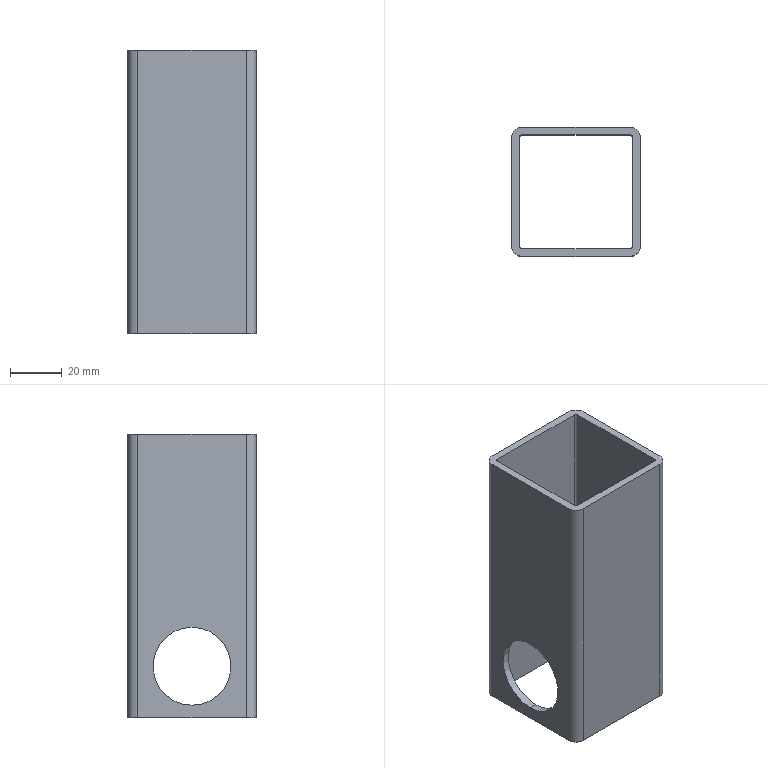Part | SolidWorks | features ExtruThin 1, ICE 1 | 1 solid | 22 faces | box 50 x 50 x 110 mm | volume 56326 mm3 | cylinder 12 | plane 10 | commonest cylinder face diameters 2 x4 8 x4 30.2 x4
STEP:
#1=CARTESIAN_POINT('',(22.,0.,4.9));
#2=VERTEX_POINT('',#1);
#3=CARTESIAN_POINT('',(22.,0.,35.1));
#4=VERTEX_POINT('',#3);
#5=CARTESIAN_POINT('',(22.,0.,20.));
#6=DIRECTION('',(-1.,0.,0.));
#7=DIRECTION('',(0.,0.,1.));
#8=AXIS2_PLACEMENT_3D('',#5,#6,#7);
#9=CIRCLE('',#8,15.1);
#10=EDGE_CURVE('',#2,#4,#9,.T.);
#11=ORIENTED_EDGE('',*,*,#10,.T.);
#12=CARTESIAN_POINT('',(25.,0.,35.1));
#13=VERTEX_POINT('',#12);
#14=CARTESIAN_POINT('',(-25.,0.,35.1));
#15=DIRECTION('',(1.,0.,0.));
#16=VECTOR('',#15,1000.);
#17=LINE('',#14,#16);
#18=EDGE_CURVE('',#4,#13,#17,.T.);
#19=ORIENTED_EDGE('',*,*,#18,.T.);
#20=CARTESIAN_POINT('',(25.,0.,4.9));
#21=VERTEX_POINT('',#20);
#22=CARTESIAN_POINT('',(25.,0.,20.));
#23=DIRECTION('',(1.,0.,0.));
#24=DIRECTION('',(0.,0.,-1.));
#25=AXIS2_PLACEMENT_3D('',#22,#23,#24);
#26=CIRCLE('',#25,15.1);
#27=EDGE_CURVE('',#13,#21,#26,.T.);
#28=ORIENTED_EDGE('',*,*,#27,.T.);
#29=CARTESIAN_POINT('',(-25.,0.,4.9));
#30=DIRECTION('',(1.,0.,0.));
#31=VECTOR('',#30,1000.);
#32=LINE('',#29,#31);
#33=EDGE_CURVE('',#2,#21,#32,.T.);
#34=ORIENTED_EDGE('',*,*,#33,.F.);
#35=EDGE_LOOP('',(#11,#19,#28,#34));
#36=FACE_OUTER_BOUND('',#35,.T.);
#37=CARTESIAN_POINT('',(-25.,0.,20.));
#38=DIRECTION('',(1.,0.,0.));
#39=DIRECTION('',(0.,0.,-1.));
#40=AXIS2_PLACEMENT_3D('',#37,#38,#39);
#41=CYLINDRICAL_SURFACE('',#40,15.1);
#42=ADVANCED_FACE('',(#36),#41,.F.);
#43=CARTESIAN_POINT('',(-25.,0.,35.1));
#44=VERTEX_POINT('',#43);
#45=CARTESIAN_POINT('',(-25.,0.,4.9));
#46=VERTEX_POINT('',#45);
#47=CARTESIAN_POINT('',(-25.,0.,20.));
#48=DIRECTION('',(1.,0.,0.));
#49=DIRECTION('',(0.,0.,-1.));
#50=AXIS2_PLACEMENT_3D('',#47,#48,#49);
#51=CIRCLE('',#50,15.1);
#52=EDGE_CURVE('',#44,#46,#51,.T.);
#53=ORIENTED_EDGE('',*,*,#52,.F.);
#54=CARTESIAN_POINT('',(-22.,0.,35.1));
#55=VERTEX_POINT('',#54);
#56=CARTESIAN_POINT('',(-25.,0.,35.1));
#57=DIRECTION('',(1.,0.,0.));
#58=VECTOR('',#57,1000.);
#59=LINE('',#56,#58);
#60=EDGE_CURVE('',#44,#55,#59,.T.);
#61=ORIENTED_EDGE('',*,*,#60,.T.);
#62=CARTESIAN_POINT('',(-22.,0.,4.9));
#63=VERTEX_POINT('',#62);
#64=CARTESIAN_POINT('',(-22.,0.,20.));
#65=DIRECTION('',(1.,0.,0.));
#66=DIRECTION('',(0.,0.,-1.));
#67=AXIS2_PLACEMENT_3D('',#64,#65,#66);
#68=CIRCLE('',#67,15.1);
#69=EDGE_CURVE('',#55,#63,#68,.T.);
#70=ORIENTED_EDGE('',*,*,#69,.T.);
#71=CARTESIAN_POINT('',(-25.,0.,4.9));
#72=DIRECTION('',(1.,0.,0.));
#73=VECTOR('',#72,1000.);
#74=LINE('',#71,#73);
#75=EDGE_CURVE('',#46,#63,#74,.T.);
#76=ORIENTED_EDGE('',*,*,#75,.F.);
#77=EDGE_LOOP('',(#53,#61,#70,#76));
#78=FACE_OUTER_BOUND('',#77,.T.);
#79=CARTESIAN_POINT('',(-25.,0.,20.));
#80=DIRECTION('',(1.,0.,0.));
#81=DIRECTION('',(0.,0.,-1.));
#82=AXIS2_PLACEMENT_3D('',#79,#80,#81);
#83=CYLINDRICAL_SURFACE('',#82,15.1);
#84=ADVANCED_FACE('',(#78),#83,.F.);
#85=CARTESIAN_POINT('',(-25.,-21.,110.));
#86=VERTEX_POINT('',#85);
#87=CARTESIAN_POINT('',(-21.,-25.,110.));
#88=VERTEX_POINT('',#87);
#89=CARTESIAN_POINT('',(-21.,-21.,110.));
#90=DIRECTION('',(0.,0.,1.));
#91=DIRECTION('',(-1.,0.,0.));
#92=AXIS2_PLACEMENT_3D('',#89,#90,#91);
#93=CIRCLE('',#92,4.);
#94=EDGE_CURVE('',#86,#88,#93,.T.);
#95=ORIENTED_EDGE('',*,*,#94,.T.);
#96=CARTESIAN_POINT('',(21.,-25.,110.));
#97=VERTEX_POINT('',#96);
#98=CARTESIAN_POINT('',(-21.,-25.,110.));
#99=DIRECTION('',(1.,0.,0.));
#100=VECTOR('',#99,1000.);
#101=LINE('',#98,#100);
#102=EDGE_CURVE('',#88,#97,#101,.T.);
#103=ORIENTED_EDGE('',*,*,#102,.T.);
#104=CARTESIAN_POINT('',(25.,-21.,110.));
#105=VERTEX_POINT('',#104);
#106=CARTESIAN_POINT('',(21.,-21.,110.));
#107=DIRECTION('',(0.,0.,1.));
#108=DIRECTION('',(1.,0.,0.));
#109=AXIS2_PLACEMENT_3D('',#106,#107,#108);
#110=CIRCLE('',#109,4.);
#111=EDGE_CURVE('',#97,#105,#110,.T.);
#112=ORIENTED_EDGE('',*,*,#111,.T.);
#113=CARTESIAN_POINT('',(25.,21.,110.));
#114=VERTEX_POINT('',#113);
#115=CARTESIAN_POINT('',(25.,-21.,110.));
#116=DIRECTION('',(0.,1.,0.));
#117=VECTOR('',#116,1000.);
#118=LINE('',#115,#117);
#119=EDGE_CURVE('',#105,#114,#118,.T.);
#120=ORIENTED_EDGE('',*,*,#119,.T.);
#121=CARTESIAN_POINT('',(21.,25.,110.));
#122=VERTEX_POINT('',#121);
#123=CARTESIAN_POINT('',(21.,21.,110.));
#124=DIRECTION('',(0.,0.,1.));
#125=DIRECTION('',(-1.,0.,0.));
#126=AXIS2_PLACEMENT_3D('',#123,#124,#125);
#127=CIRCLE('',#126,4.);
#128=EDGE_CURVE('',#114,#122,#127,.T.);
#129=ORIENTED_EDGE('',*,*,#128,.T.);
#130=CARTESIAN_POINT('',(-21.,25.,110.));
#131=VERTEX_POINT('',#130);
#132=CARTESIAN_POINT('',(-21.,25.,110.));
#133=DIRECTION('',(-1.,0.,0.));
#134=VECTOR('',#133,1000.);
#135=LINE('',#132,#134);
#136=EDGE_CURVE('',#122,#131,#135,.T.);
#137=ORIENTED_EDGE('',*,*,#136,.T.);
#138=CARTESIAN_POINT('',(-25.,21.,110.));
#139=VERTEX_POINT('',#138);
#140=CARTESIAN_POINT('',(-21.,21.,110.));
#141=DIRECTION('',(0.,0.,1.));
#142=DIRECTION('',(-1.,0.,0.));
#143=AXIS2_PLACEMENT_3D('',#140,#141,#142);
#144=CIRCLE('',#143,4.);
#145=EDGE_CURVE('',#131,#139,#144,.T.);
#146=ORIENTED_EDGE('',*,*,#145,.T.);
#147=CARTESIAN_POINT('',(-25.,-21.,110.));
#148=DIRECTION('',(0.,-1.,0.));
#149=VECTOR('',#148,1000.);
#150=LINE('',#147,#149);
#151=EDGE_CURVE('',#139,#86,#150,.T.);
#152=ORIENTED_EDGE('',*,*,#151,.T.);
#153=EDGE_LOOP('',(#95,#103,#112,#120,#129,#137,#146,#152));
#154=FACE_OUTER_BOUND('',#153,.T.);
#155=CARTESIAN_POINT('',(-21.,-22.,110.));
#156=VERTEX_POINT('',#155);
#157=CARTESIAN_POINT('',(21.,-22.,110.));
#158=VERTEX_POINT('',#157);
#159=CARTESIAN_POINT('',(-21.,-22.,110.));
#160=DIRECTION('',(1.,0.,0.));
#161=VECTOR('',#160,1000.);
#162=LINE('',#159,#161);
#163=EDGE_CURVE('',#156,#158,#162,.T.);
#164=ORIENTED_EDGE('',*,*,#163,.F.);
#165=CARTESIAN_POINT('',(-22.,-21.,110.));
#166=VERTEX_POINT('',#165);
#167=CARTESIAN_POINT('',(-21.,-21.,110.));
#168=DIRECTION('',(0.,0.,1.));
#169=DIRECTION('',(-1.,0.,0.));
#170=AXIS2_PLACEMENT_3D('',#167,#168,#169);
#171=CIRCLE('',#170,1.);
#172=EDGE_CURVE('',#166,#156,#171,.T.);
#173=ORIENTED_EDGE('',*,*,#172,.F.);
#174=CARTESIAN_POINT('',(-22.,21.,110.));
#175=VERTEX_POINT('',#174);
#176=CARTESIAN_POINT('',(-22.,-21.,110.));
#177=DIRECTION('',(0.,-1.,0.));
#178=VECTOR('',#177,1000.);
#179=LINE('',#176,#178);
#180=EDGE_CURVE('',#175,#166,#179,.T.);
#181=ORIENTED_EDGE('',*,*,#180,.F.);
#182=CARTESIAN_POINT('',(-21.,22.,110.));
#183=VERTEX_POINT('',#182);
#184=CARTESIAN_POINT('',(-21.,21.,110.));
#185=DIRECTION('',(0.,0.,1.));
#186=DIRECTION('',(-1.,0.,0.));
#187=AXIS2_PLACEMENT_3D('',#184,#185,#186);
#188=CIRCLE('',#187,1.);
#189=EDGE_CURVE('',#183,#175,#188,.T.);
#190=ORIENTED_EDGE('',*,*,#189,.F.);
#191=CARTESIAN_POINT('',(21.,22.,110.));
#192=VERTEX_POINT('',#191);
#193=CARTESIAN_POINT('',(-21.,22.,110.));
#194=DIRECTION('',(-1.,0.,0.));
#195=VECTOR('',#194,1000.);
#196=LINE('',#193,#195);
#197=EDGE_CURVE('',#192,#183,#196,.T.);
#198=ORIENTED_EDGE('',*,*,#197,.F.);
#199=CARTESIAN_POINT('',(22.,21.,110.));
#200=VERTEX_POINT('',#199);
#201=CARTESIAN_POINT('',(21.,21.,110.));
#202=DIRECTION('',(0.,0.,1.));
#203=DIRECTION('',(-1.,0.,0.));
#204=AXIS2_PLACEMENT_3D('',#201,#202,#203);
#205=CIRCLE('',#204,1.);
#206=EDGE_CURVE('',#200,#192,#205,.T.);
#207=ORIENTED_EDGE('',*,*,#206,.F.);
#208=CARTESIAN_POINT('',(22.,-21.,110.));
#209=VERTEX_POINT('',#208);
#210=CARTESIAN_POINT('',(22.,-21.,110.));
#211=DIRECTION('',(0.,1.,0.));
#212=VECTOR('',#211,1000.);
#213=LINE('',#210,#212);
#214=EDGE_CURVE('',#209,#200,#213,.T.);
#215=ORIENTED_EDGE('',*,*,#214,.F.);
#216=CARTESIAN_POINT('',(21.,-21.,110.));
#217=DIRECTION('',(0.,0.,1.));
#218=DIRECTION('',(-1.,0.,0.));
#219=AXIS2_PLACEMENT_3D('',#216,#217,#218);
#220=CIRCLE('',#219,1.);
#221=EDGE_CURVE('',#158,#209,#220,.T.);
#222=ORIENTED_EDGE('',*,*,#221,.F.);
#223=EDGE_LOOP('',(#164,#173,#181,#190,#198,#207,#215,#222));
#224=FACE_BOUND('',#223,.T.);
#225=CARTESIAN_POINT('',(-21.,-21.,110.));
#226=DIRECTION('',(0.,0.,1.));
#227=DIRECTION('',(1.,0.,0.));
#228=AXIS2_PLACEMENT_3D('',#225,#226,#227);
#229=PLANE('',#228);
#230=ADVANCED_FACE('',(#154,#224),#229,.T.);
#231=CARTESIAN_POINT('',(-25.,-21.,0.));
#232=VERTEX_POINT('',#231);
#233=CARTESIAN_POINT('',(-21.,-25.,0.));
#234=VERTEX_POINT('',#233);
#235=CARTESIAN_POINT('',(-21.,-21.,0.));
#236=DIRECTION('',(0.,0.,1.));
#237=DIRECTION('',(-1.,0.,0.));
#238=AXIS2_PLACEMENT_3D('',#235,#236,#237);
#239=CIRCLE('',#238,4.);
#240=EDGE_CURVE('',#232,#234,#239,.T.);
#241=ORIENTED_EDGE('',*,*,#240,.F.);
#242=CARTESIAN_POINT('',(-25.,21.,0.));
#243=VERTEX_POINT('',#242);
#244=CARTESIAN_POINT('',(-25.,-21.,0.));
#245=DIRECTION('',(0.,-1.,0.));
#246=VECTOR('',#245,1000.);
#247=LINE('',#244,#246);
#248=EDGE_CURVE('',#243,#232,#247,.T.);
#249=ORIENTED_EDGE('',*,*,#248,.F.);
#250=CARTESIAN_POINT('',(-21.,25.,0.));
#251=VERTEX_POINT('',#250);
#252=CARTESIAN_POINT('',(-21.,21.,0.));
#253=DIRECTION('',(0.,0.,1.));
#254=DIRECTION('',(-1.,0.,0.));
#255=AXIS2_PLACEMENT_3D('',#252,#253,#254);
#256=CIRCLE('',#255,4.);
#257=EDGE_CURVE('',#251,#243,#256,.T.);
#258=ORIENTED_EDGE('',*,*,#257,.F.);
#259=CARTESIAN_POINT('',(21.,25.,0.));
#260=VERTEX_POINT('',#259);
#261=CARTESIAN_POINT('',(-21.,25.,0.));
#262=DIRECTION('',(-1.,0.,0.));
#263=VECTOR('',#262,1000.);
#264=LINE('',#261,#263);
#265=EDGE_CURVE('',#260,#251,#264,.T.);
#266=ORIENTED_EDGE('',*,*,#265,.F.);
#267=CARTESIAN_POINT('',(25.,21.,0.));
#268=VERTEX_POINT('',#267);
#269=CARTESIAN_POINT('',(21.,21.,0.));
#270=DIRECTION('',(0.,0.,1.));
#271=DIRECTION('',(-1.,0.,0.));
#272=AXIS2_PLACEMENT_3D('',#269,#270,#271);
#273=CIRCLE('',#272,4.);
#274=EDGE_CURVE('',#268,#260,#273,.T.);
#275=ORIENTED_EDGE('',*,*,#274,.F.);
#276=CARTESIAN_POINT('',(25.,-21.,0.));
#277=VERTEX_POINT('',#276);
#278=CARTESIAN_POINT('',(25.,-21.,0.));
#279=DIRECTION('',(0.,1.,0.));
#280=VECTOR('',#279,1000.);
#281=LINE('',#278,#280);
#282=EDGE_CURVE('',#277,#268,#281,.T.);
#283=ORIENTED_EDGE('',*,*,#282,.F.);
#284=CARTESIAN_POINT('',(21.,-25.,0.));
#285=VERTEX_POINT('',#284);
#286=CARTESIAN_POINT('',(21.,-21.,0.));
#287=DIRECTION('',(0.,0.,1.));
#288=DIRECTION('',(1.,0.,0.));
#289=AXIS2_PLACEMENT_3D('',#286,#287,#288);
#290=CIRCLE('',#289,4.);
#291=EDGE_CURVE('',#285,#277,#290,.T.);
#292=ORIENTED_EDGE('',*,*,#291,.F.);
#293=CARTESIAN_POINT('',(-21.,-25.,0.));
#294=DIRECTION('',(1.,0.,0.));
#295=VECTOR('',#294,1000.);
#296=LINE('',#293,#295);
#297=EDGE_CURVE('',#234,#285,#296,.T.);
#298=ORIENTED_EDGE('',*,*,#297,.F.);
#299=EDGE_LOOP('',(#241,#249,#258,#266,#275,#283,#292,#298));
#300=FACE_OUTER_BOUND('',#299,.T.);
#301=CARTESIAN_POINT('',(-22.,-21.,0.));
#302=VERTEX_POINT('',#301);
#303=CARTESIAN_POINT('',(-21.,-22.,0.));
#304=VERTEX_POINT('',#303);
#305=CARTESIAN_POINT('',(-21.,-21.,0.));
#306=DIRECTION('',(0.,0.,1.));
#307=DIRECTION('',(-1.,0.,0.));
#308=AXIS2_PLACEMENT_3D('',#305,#306,#307);
#309=CIRCLE('',#308,1.);
#310=EDGE_CURVE('',#302,#304,#309,.T.);
#311=ORIENTED_EDGE('',*,*,#310,.T.);
#312=CARTESIAN_POINT('',(21.,-22.,0.));
#313=VERTEX_POINT('',#312);
#314=CARTESIAN_POINT('',(-21.,-22.,0.));
#315=DIRECTION('',(1.,0.,0.));
#316=VECTOR('',#315,1000.);
#317=LINE('',#314,#316);
#318=EDGE_CURVE('',#304,#313,#317,.T.);
#319=ORIENTED_EDGE('',*,*,#318,.T.);
#320=CARTESIAN_POINT('',(22.,-21.,0.));
#321=VERTEX_POINT('',#320);
#322=CARTESIAN_POINT('',(21.,-21.,0.));
#323=DIRECTION('',(0.,0.,1.));
#324=DIRECTION('',(-1.,0.,0.));
#325=AXIS2_PLACEMENT_3D('',#322,#323,#324);
#326=CIRCLE('',#325,1.);
#327=EDGE_CURVE('',#313,#321,#326,.T.);
#328=ORIENTED_EDGE('',*,*,#327,.T.);
#329=CARTESIAN_POINT('',(22.,21.,0.));
#330=VERTEX_POINT('',#329);
#331=CARTESIAN_POINT('',(22.,-21.,0.));
#332=DIRECTION('',(0.,1.,0.));
#333=VECTOR('',#332,1000.);
#334=LINE('',#331,#333);
#335=EDGE_CURVE('',#321,#330,#334,.T.);
#336=ORIENTED_EDGE('',*,*,#335,.T.);
#337=CARTESIAN_POINT('',(21.,22.,0.));
#338=VERTEX_POINT('',#337);
#339=CARTESIAN_POINT('',(21.,21.,0.));
#340=DIRECTION('',(0.,0.,1.));
#341=DIRECTION('',(-1.,0.,0.));
#342=AXIS2_PLACEMENT_3D('',#339,#340,#341);
#343=CIRCLE('',#342,1.);
#344=EDGE_CURVE('',#330,#338,#343,.T.);
#345=ORIENTED_EDGE('',*,*,#344,.T.);
#346=CARTESIAN_POINT('',(-21.,22.,0.));
#347=VERTEX_POINT('',#346);
#348=CARTESIAN_POINT('',(-21.,22.,0.));
#349=DIRECTION('',(-1.,0.,0.));
#350=VECTOR('',#349,1000.);
#351=LINE('',#348,#350);
#352=EDGE_CURVE('',#338,#347,#351,.T.);
#353=ORIENTED_EDGE('',*,*,#352,.T.);
#354=CARTESIAN_POINT('',(-22.,21.,0.));
#355=VERTEX_POINT('',#354);
#356=CARTESIAN_POINT('',(-21.,21.,0.));
#357=DIRECTION('',(0.,0.,1.));
#358=DIRECTION('',(-1.,0.,0.));
#359=AXIS2_PLACEMENT_3D('',#356,#357,#358);
#360=CIRCLE('',#359,1.);
#361=EDGE_CURVE('',#347,#355,#360,.T.);
#362=ORIENTED_EDGE('',*,*,#361,.T.);
#363=CARTESIAN_POINT('',(-22.,-21.,0.));
#364=DIRECTION('',(0.,-1.,0.));
#365=VECTOR('',#364,1000.);
#366=LINE('',#363,#365);
#367=EDGE_CURVE('',#355,#302,#366,.T.);
#368=ORIENTED_EDGE('',*,*,#367,.T.);
#369=EDGE_LOOP('',(#311,#319,#328,#336,#345,#353,#362,#368));
#370=FACE_BOUND('',#369,.T.);
#371=CARTESIAN_POINT('',(-21.,-21.,0.));
#372=DIRECTION('',(0.,0.,1.));
#373=DIRECTION('',(1.,0.,0.));
#374=AXIS2_PLACEMENT_3D('',#371,#372,#373);
#375=PLANE('',#374);
#376=ADVANCED_FACE('',(#300,#370),#375,.F.);
#377=ORIENTED_EDGE('',*,*,#240,.T.);
#378=CARTESIAN_POINT('',(-21.,-25.,110.));
#379=DIRECTION('',(0.,0.,-1.));
#380=VECTOR('',#379,1000.);
#381=LINE('',#378,#380);
#382=EDGE_CURVE('',#88,#234,#381,.T.);
#383=ORIENTED_EDGE('',*,*,#382,.F.);
#384=ORIENTED_EDGE('',*,*,#94,.F.);
#385=CARTESIAN_POINT('',(-25.,-21.,110.));
#386=DIRECTION('',(0.,0.,-1.));
#387=VECTOR('',#386,1000.);
#388=LINE('',#385,#387);
#389=EDGE_CURVE('',#86,#232,#388,.T.);
#390=ORIENTED_EDGE('',*,*,#389,.T.);
#391=EDGE_LOOP('',(#377,#383,#384,#390));
#392=FACE_OUTER_BOUND('',#391,.T.);
#393=CARTESIAN_POINT('',(-21.,-21.,110.));
#394=DIRECTION('',(0.,0.,-1.));
#395=DIRECTION('',(-1.,0.,0.));
#396=AXIS2_PLACEMENT_3D('',#393,#394,#395);
#397=CYLINDRICAL_SURFACE('',#396,4.);
#398=ADVANCED_FACE('',(#392),#397,.T.);
#399=ORIENTED_EDGE('',*,*,#297,.T.);
#400=CARTESIAN_POINT('',(21.,-25.,110.));
#401=DIRECTION('',(0.,0.,-1.));
#402=VECTOR('',#401,1000.);
#403=LINE('',#400,#402);
#404=EDGE_CURVE('',#97,#285,#403,.T.);
#405=ORIENTED_EDGE('',*,*,#404,.F.);
#406=ORIENTED_EDGE('',*,*,#102,.F.);
#407=ORIENTED_EDGE('',*,*,#382,.T.);
#408=EDGE_LOOP('',(#399,#405,#406,#407));
#409=FACE_OUTER_BOUND('',#408,.T.);
#410=CARTESIAN_POINT('',(-21.,-25.,110.));
#411=DIRECTION('',(0.,1.,0.));
#412=DIRECTION('',(0.,0.,1.));
#413=AXIS2_PLACEMENT_3D('',#410,#411,#412);
#414=PLANE('',#413);
#415=ADVANCED_FACE('',(#409),#414,.F.);
#416=ORIENTED_EDGE('',*,*,#291,.T.);
#417=CARTESIAN_POINT('',(25.,-21.,110.));
#418=DIRECTION('',(0.,0.,-1.));
#419=VECTOR('',#418,1000.);
#420=LINE('',#417,#419);
#421=EDGE_CURVE('',#105,#277,#420,.T.);
#422=ORIENTED_EDGE('',*,*,#421,.F.);
#423=ORIENTED_EDGE('',*,*,#111,.F.);
#424=ORIENTED_EDGE('',*,*,#404,.T.);
#425=EDGE_LOOP('',(#416,#422,#423,#424));
#426=FACE_OUTER_BOUND('',#425,.T.);
#427=CARTESIAN_POINT('',(21.,-21.,110.));
#428=DIRECTION('',(0.,0.,-1.));
#429=DIRECTION('',(-1.,0.,0.));
#430=AXIS2_PLACEMENT_3D('',#427,#428,#429);
#431=CYLINDRICAL_SURFACE('',#430,4.);
#432=ADVANCED_FACE('',(#426),#431,.T.);
#433=CARTESIAN_POINT('',(25.,0.,20.));
#434=DIRECTION('',(1.,0.,0.));
#435=DIRECTION('',(0.,0.,-1.));
#436=AXIS2_PLACEMENT_3D('',#433,#434,#435);
#437=CIRCLE('',#436,15.1);
#438=EDGE_CURVE('',#21,#13,#437,.T.);
#439=ORIENTED_EDGE('',*,*,#438,.F.);
#440=ORIENTED_EDGE('',*,*,#27,.F.);
#441=EDGE_LOOP('',(#439,#440));
#442=FACE_BOUND('',#441,.T.);
#443=ORIENTED_EDGE('',*,*,#282,.T.);
#444=CARTESIAN_POINT('',(25.,21.,110.));
#445=DIRECTION('',(0.,0.,-1.));
#446=VECTOR('',#445,1000.);
#447=LINE('',#444,#446);
#448=EDGE_CURVE('',#114,#268,#447,.T.);
#449=ORIENTED_EDGE('',*,*,#448,.F.);
#450=ORIENTED_EDGE('',*,*,#119,.F.);
#451=ORIENTED_EDGE('',*,*,#421,.T.);
#452=EDGE_LOOP('',(#443,#449,#450,#451));
#453=FACE_OUTER_BOUND('',#452,.T.);
#454=CARTESIAN_POINT('',(25.,-21.,110.));
#455=DIRECTION('',(-1.,0.,0.));
#456=DIRECTION('',(0.,0.,1.));
#457=AXIS2_PLACEMENT_3D('',#454,#455,#456);
#458=PLANE('',#457);
#459=ADVANCED_FACE('',(#442,#453),#458,.F.);
#460=ORIENTED_EDGE('',*,*,#274,.T.);
#461=CARTESIAN_POINT('',(21.,25.,110.));
#462=DIRECTION('',(0.,0.,-1.));
#463=VECTOR('',#462,1000.);
#464=LINE('',#461,#463);
#465=EDGE_CURVE('',#122,#260,#464,.T.);
#466=ORIENTED_EDGE('',*,*,#465,.F.);
#467=ORIENTED_EDGE('',*,*,#128,.F.);
#468=ORIENTED_EDGE('',*,*,#448,.T.);
#469=EDGE_LOOP('',(#460,#466,#467,#468));
#470=FACE_OUTER_BOUND('',#469,.T.);
#471=CARTESIAN_POINT('',(21.,21.,110.));
#472=DIRECTION('',(0.,0.,-1.));
#473=DIRECTION('',(-1.,0.,0.));
#474=AXIS2_PLACEMENT_3D('',#471,#472,#473);
#475=CYLINDRICAL_SURFACE('',#474,4.);
#476=ADVANCED_FACE('',(#470),#475,.T.);
#477=ORIENTED_EDGE('',*,*,#265,.T.);
#478=CARTESIAN_POINT('',(-21.,25.,110.));
#479=DIRECTION('',(0.,0.,-1.));
#480=VECTOR('',#479,1000.);
#481=LINE('',#478,#480);
#482=EDGE_CURVE('',#131,#251,#481,.T.);
#483=ORIENTED_EDGE('',*,*,#482,.F.);
#484=ORIENTED_EDGE('',*,*,#136,.F.);
#485=ORIENTED_EDGE('',*,*,#465,.T.);
#486=EDGE_LOOP('',(#477,#483,#484,#485));
#487=FACE_OUTER_BOUND('',#486,.T.);
#488=CARTESIAN_POINT('',(-21.,25.,110.));
#489=DIRECTION('',(0.,-1.,0.));
#490=DIRECTION('',(0.,0.,-1.));
#491=AXIS2_PLACEMENT_3D('',#488,#489,#490);
#492=PLANE('',#491);
#493=ADVANCED_FACE('',(#487),#492,.F.);
#494=ORIENTED_EDGE('',*,*,#257,.T.);
#495=CARTESIAN_POINT('',(-25.,21.,110.));
#496=DIRECTION('',(0.,0.,-1.));
#497=VECTOR('',#496,1000.);
#498=LINE('',#495,#497);
#499=EDGE_CURVE('',#139,#243,#498,.T.);
#500=ORIENTED_EDGE('',*,*,#499,.F.);
#501=ORIENTED_EDGE('',*,*,#145,.F.);
#502=ORIENTED_EDGE('',*,*,#482,.T.);
#503=EDGE_LOOP('',(#494,#500,#501,#502));
#504=FACE_OUTER_BOUND('',#503,.T.);
#505=CARTESIAN_POINT('',(-21.,21.,110.));
#506=DIRECTION('',(0.,0.,-1.));
#507=DIRECTION('',(-1.,0.,0.));
#508=AXIS2_PLACEMENT_3D('',#505,#506,#507);
#509=CYLINDRICAL_SURFACE('',#508,4.);
#510=ADVANCED_FACE('',(#504),#509,.T.);
#511=CARTESIAN_POINT('',(-25.,0.,20.));
#512=DIRECTION('',(1.,0.,0.));
#513=DIRECTION('',(0.,0.,-1.));
#514=AXIS2_PLACEMENT_3D('',#511,#512,#513);
#515=CIRCLE('',#514,15.1);
#516=EDGE_CURVE('',#46,#44,#515,.T.);
#517=ORIENTED_EDGE('',*,*,#516,.T.);
#518=ORIENTED_EDGE('',*,*,#52,.T.);
#519=EDGE_LOOP('',(#517,#518));
#520=FACE_BOUND('',#519,.T.);
#521=ORIENTED_EDGE('',*,*,#248,.T.);
#522=ORIENTED_EDGE('',*,*,#389,.F.);
#523=ORIENTED_EDGE('',*,*,#151,.F.);
#524=ORIENTED_EDGE('',*,*,#499,.T.);
#525=EDGE_LOOP('',(#521,#522,#523,#524));
#526=FACE_OUTER_BOUND('',#525,.T.);
#527=CARTESIAN_POINT('',(-25.,-21.,110.));
#528=DIRECTION('',(1.,0.,0.));
#529=DIRECTION('',(0.,0.,-1.));
#530=AXIS2_PLACEMENT_3D('',#527,#528,#529);
#531=PLANE('',#530);
#532=ADVANCED_FACE('',(#520,#526),#531,.F.);
#533=ORIENTED_EDGE('',*,*,#310,.F.);
#534=CARTESIAN_POINT('',(-22.,-21.,110.));
#535=DIRECTION('',(0.,0.,-1.));
#536=VECTOR('',#535,1000.);
#537=LINE('',#534,#536);
#538=EDGE_CURVE('',#166,#302,#537,.T.);
#539=ORIENTED_EDGE('',*,*,#538,.F.);
#540=ORIENTED_EDGE('',*,*,#172,.T.);
#541=CARTESIAN_POINT('',(-21.,-22.,110.));
#542=DIRECTION('',(0.,0.,-1.));
#543=VECTOR('',#542,1000.);
#544=LINE('',#541,#543);
#545=EDGE_CURVE('',#156,#304,#544,.T.);
#546=ORIENTED_EDGE('',*,*,#545,.T.);
#547=EDGE_LOOP('',(#533,#539,#540,#546));
#548=FACE_OUTER_BOUND('',#547,.T.);
#549=CARTESIAN_POINT('',(-21.,-21.,110.));
#550=DIRECTION('',(0.,0.,-1.));
#551=DIRECTION('',(-1.,0.,0.));
#552=AXIS2_PLACEMENT_3D('',#549,#550,#551);
#553=CYLINDRICAL_SURFACE('',#552,1.);
#554=ADVANCED_FACE('',(#548),#553,.F.);
#555=ORIENTED_EDGE('',*,*,#318,.F.);
#556=ORIENTED_EDGE('',*,*,#545,.F.);
#557=ORIENTED_EDGE('',*,*,#163,.T.);
#558=CARTESIAN_POINT('',(21.,-22.,110.));
#559=DIRECTION('',(0.,0.,-1.));
#560=VECTOR('',#559,1000.);
#561=LINE('',#558,#560);
#562=EDGE_CURVE('',#158,#313,#561,.T.);
#563=ORIENTED_EDGE('',*,*,#562,.T.);
#564=EDGE_LOOP('',(#555,#556,#557,#563));
#565=FACE_OUTER_BOUND('',#564,.T.);
#566=CARTESIAN_POINT('',(-21.,-22.,110.));
#567=DIRECTION('',(0.,1.,0.));
#568=DIRECTION('',(0.,0.,1.));
#569=AXIS2_PLACEMENT_3D('',#566,#567,#568);
#570=PLANE('',#569);
#571=ADVANCED_FACE('',(#565),#570,.T.);
#572=ORIENTED_EDGE('',*,*,#327,.F.);
#573=ORIENTED_EDGE('',*,*,#562,.F.);
#574=ORIENTED_EDGE('',*,*,#221,.T.);
#575=CARTESIAN_POINT('',(22.,-21.,110.));
#576=DIRECTION('',(0.,0.,-1.));
#577=VECTOR('',#576,1000.);
#578=LINE('',#575,#577);
#579=EDGE_CURVE('',#209,#321,#578,.T.);
#580=ORIENTED_EDGE('',*,*,#579,.T.);
#581=EDGE_LOOP('',(#572,#573,#574,#580));
#582=FACE_OUTER_BOUND('',#581,.T.);
#583=CARTESIAN_POINT('',(21.,-21.,110.));
#584=DIRECTION('',(0.,0.,-1.));
#585=DIRECTION('',(-1.,0.,0.));
#586=AXIS2_PLACEMENT_3D('',#583,#584,#585);
#587=CYLINDRICAL_SURFACE('',#586,1.);
#588=ADVANCED_FACE('',(#582),#587,.F.);
#589=ORIENTED_EDGE('',*,*,#10,.F.);
#590=CARTESIAN_POINT('',(22.,0.,20.));
#591=DIRECTION('',(-1.,0.,0.));
#592=DIRECTION('',(0.,0.,1.));
#593=AXIS2_PLACEMENT_3D('',#590,#591,#592);
#594=CIRCLE('',#593,15.1);
#595=EDGE_CURVE('',#4,#2,#594,.T.);
#596=ORIENTED_EDGE('',*,*,#595,.F.);
#597=EDGE_LOOP('',(#589,#596));
#598=FACE_BOUND('',#597,.T.);
#599=ORIENTED_EDGE('',*,*,#335,.F.);
#600=ORIENTED_EDGE('',*,*,#579,.F.);
#601=ORIENTED_EDGE('',*,*,#214,.T.);
#602=CARTESIAN_POINT('',(22.,21.,110.));
#603=DIRECTION('',(0.,0.,-1.));
#604=VECTOR('',#603,1000.);
#605=LINE('',#602,#604);
#606=EDGE_CURVE('',#200,#330,#605,.T.);
#607=ORIENTED_EDGE('',*,*,#606,.T.);
#608=EDGE_LOOP('',(#599,#600,#601,#607));
#609=FACE_OUTER_BOUND('',#608,.T.);
#610=CARTESIAN_POINT('',(22.,-21.,110.));
#611=DIRECTION('',(-1.,0.,0.));
#612=DIRECTION('',(0.,0.,1.));
#613=AXIS2_PLACEMENT_3D('',#610,#611,#612);
#614=PLANE('',#613);
#615=ADVANCED_FACE('',(#598,#609),#614,.T.);
#616=ORIENTED_EDGE('',*,*,#344,.F.);
#617=ORIENTED_EDGE('',*,*,#606,.F.);
#618=ORIENTED_EDGE('',*,*,#206,.T.);
#619=CARTESIAN_POINT('',(21.,22.,110.));
#620=DIRECTION('',(0.,0.,-1.));
#621=VECTOR('',#620,1000.);
#622=LINE('',#619,#621);
#623=EDGE_CURVE('',#192,#338,#622,.T.);
#624=ORIENTED_EDGE('',*,*,#623,.T.);
#625=EDGE_LOOP('',(#616,#617,#618,#624));
#626=FACE_OUTER_BOUND('',#625,.T.);
#627=CARTESIAN_POINT('',(21.,21.,110.));
#628=DIRECTION('',(0.,0.,-1.));
#629=DIRECTION('',(-1.,0.,0.));
#630=AXIS2_PLACEMENT_3D('',#627,#628,#629);
#631=CYLINDRICAL_SURFACE('',#630,1.);
#632=ADVANCED_FACE('',(#626),#631,.F.);
#633=ORIENTED_EDGE('',*,*,#352,.F.);
#634=ORIENTED_EDGE('',*,*,#623,.F.);
#635=ORIENTED_EDGE('',*,*,#197,.T.);
#636=CARTESIAN_POINT('',(-21.,22.,110.));
#637=DIRECTION('',(0.,0.,-1.));
#638=VECTOR('',#637,1000.);
#639=LINE('',#636,#638);
#640=EDGE_CURVE('',#183,#347,#639,.T.);
#641=ORIENTED_EDGE('',*,*,#640,.T.);
#642=EDGE_LOOP('',(#633,#634,#635,#641));
#643=FACE_OUTER_BOUND('',#642,.T.);
#644=CARTESIAN_POINT('',(-21.,22.,110.));
#645=DIRECTION('',(0.,-1.,0.));
#646=DIRECTION('',(0.,0.,-1.));
#647=AXIS2_PLACEMENT_3D('',#644,#645,#646);
#648=PLANE('',#647);
#649=ADVANCED_FACE('',(#643),#648,.T.);
#650=ORIENTED_EDGE('',*,*,#361,.F.);
#651=ORIENTED_EDGE('',*,*,#640,.F.);
#652=ORIENTED_EDGE('',*,*,#189,.T.);
#653=CARTESIAN_POINT('',(-22.,21.,110.));
#654=DIRECTION('',(0.,0.,-1.));
#655=VECTOR('',#654,1000.);
#656=LINE('',#653,#655);
#657=EDGE_CURVE('',#175,#355,#656,.T.);
#658=ORIENTED_EDGE('',*,*,#657,.T.);
#659=EDGE_LOOP('',(#650,#651,#652,#658));
#660=FACE_OUTER_BOUND('',#659,.T.);
#661=CARTESIAN_POINT('',(-21.,21.,110.));
#662=DIRECTION('',(0.,0.,-1.));
#663=DIRECTION('',(-1.,0.,0.));
#664=AXIS2_PLACEMENT_3D('',#661,#662,#663);
#665=CYLINDRICAL_SURFACE('',#664,1.);
#666=ADVANCED_FACE('',(#660),#665,.F.);
#667=CARTESIAN_POINT('',(-22.,0.,20.));
#668=DIRECTION('',(1.,0.,0.));
#669=DIRECTION('',(0.,0.,-1.));
#670=AXIS2_PLACEMENT_3D('',#667,#668,#669);
#671=CIRCLE('',#670,15.1);
#672=EDGE_CURVE('',#63,#55,#671,.T.);
#673=ORIENTED_EDGE('',*,*,#672,.F.);
#674=ORIENTED_EDGE('',*,*,#69,.F.);
#675=EDGE_LOOP('',(#673,#674));
#676=FACE_BOUND('',#675,.T.);
#677=ORIENTED_EDGE('',*,*,#367,.F.);
#678=ORIENTED_EDGE('',*,*,#657,.F.);
#679=ORIENTED_EDGE('',*,*,#180,.T.);
#680=ORIENTED_EDGE('',*,*,#538,.T.);
#681=EDGE_LOOP('',(#677,#678,#679,#680));
#682=FACE_OUTER_BOUND('',#681,.T.);
#683=CARTESIAN_POINT('',(-22.,-21.,110.));
#684=DIRECTION('',(1.,0.,0.));
#685=DIRECTION('',(0.,0.,-1.));
#686=AXIS2_PLACEMENT_3D('',#683,#684,#685);
#687=PLANE('',#686);
#688=ADVANCED_FACE('',(#676,#682),#687,.T.);
#689=ORIENTED_EDGE('',*,*,#60,.F.);
#690=ORIENTED_EDGE('',*,*,#516,.F.);
#691=ORIENTED_EDGE('',*,*,#75,.T.);
#692=ORIENTED_EDGE('',*,*,#672,.T.);
#693=EDGE_LOOP('',(#689,#690,#691,#692));
#694=FACE_OUTER_BOUND('',#693,.T.);
#695=CARTESIAN_POINT('',(-25.,0.,20.));
#696=DIRECTION('',(1.,0.,0.));
#697=DIRECTION('',(0.,0.,-1.));
#698=AXIS2_PLACEMENT_3D('',#695,#696,#697);
#699=CYLINDRICAL_SURFACE('',#698,15.1);
#700=ADVANCED_FACE('',(#694),#699,.F.);
#701=ORIENTED_EDGE('',*,*,#18,.F.);
#702=ORIENTED_EDGE('',*,*,#595,.T.);
#703=ORIENTED_EDGE('',*,*,#33,.T.);
#704=ORIENTED_EDGE('',*,*,#438,.T.);
#705=EDGE_LOOP('',(#701,#702,#703,#704));
#706=FACE_OUTER_BOUND('',#705,.T.);
#707=CARTESIAN_POINT('',(-25.,0.,20.));
#708=DIRECTION('',(1.,0.,0.));
#709=DIRECTION('',(0.,0.,-1.));
#710=AXIS2_PLACEMENT_3D('',#707,#708,#709);
#711=CYLINDRICAL_SURFACE('',#710,15.1);
#712=ADVANCED_FACE('',(#706),#711,.F.);
#713=CLOSED_SHELL('',(#42,#84,#230,#376,#398,#415,#432,#459,#476,#493,#510,#532,#554,#571,#588,#615,#632,#649,#666,#688,#700,#712));
#714=MANIFOLD_SOLID_BREP('',#713);
#715=CARTESIAN_POINT('',(0.,0.,0.));
#716=DIRECTION('',(0.,0.,1.));
#717=DIRECTION('',(1.,0.,0.));
#718=AXIS2_PLACEMENT_3D('',#715,#716,#717);
#719=(LENGTH_UNIT()NAMED_UNIT(*)SI_UNIT(.MILLI.,.METRE.));
#720=UNCERTAINTY_MEASURE_WITH_UNIT(LENGTH_MEASURE(0.00001),#719,'','');
#721=(NAMED_UNIT(*)PLANE_ANGLE_UNIT()SI_UNIT($,.RADIAN.));
#722=(NAMED_UNIT(*)SI_UNIT($,.STERADIAN.)SOLID_ANGLE_UNIT());
#723=(GEOMETRIC_REPRESENTATION_CONTEXT(3)GLOBAL_UNCERTAINTY_ASSIGNED_CONTEXT((#720))GLOBAL_UNIT_ASSIGNED_CONTEXT((#719,#721,#722))REPRESENTATION_CONTEXT('',''));
#724=ADVANCED_BREP_SHAPE_REPRESENTATION('',(#714,#718),#723);